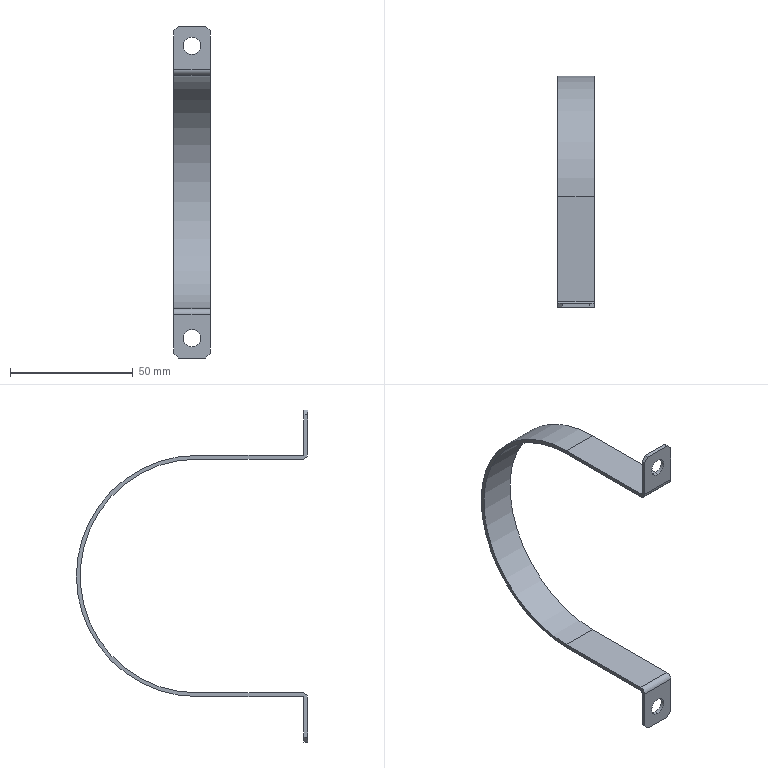Part | SolidWorks | features BaseBody 1 | 1 solid | 26 faces | box 15 x 94 x 135 mm | volume 6112 mm3 | plane 16 | cylinder 10 | commonest cylinder face diameters 7 x4 1.473 x2 4.473 x2 95 x1 98 x1
STEP:
#1=CARTESIAN_POINT('',(0.,0.,-63.));
#2=VERTEX_POINT('',#1);
#3=CARTESIAN_POINT('',(0.,0.,-56.));
#4=VERTEX_POINT('',#3);
#5=CARTESIAN_POINT('',(0.,0.,-59.5));
#6=DIRECTION('',(0.,1.,0.));
#7=DIRECTION('',(0.,0.,-1.));
#8=AXIS2_PLACEMENT_3D('',#5,#6,#7);
#9=CIRCLE('',#8,3.5);
#10=EDGE_CURVE('',#2,#4,#9,.T.);
#11=ORIENTED_EDGE('',*,*,#10,.F.);
#12=CARTESIAN_POINT('',(0.,1.5,-63.));
#13=VERTEX_POINT('',#12);
#14=CARTESIAN_POINT('',(0.,0.,-63.));
#15=DIRECTION('',(0.,1.,0.));
#16=VECTOR('',#15,1000.);
#17=LINE('',#14,#16);
#18=EDGE_CURVE('',#2,#13,#17,.T.);
#19=ORIENTED_EDGE('',*,*,#18,.T.);
#20=CARTESIAN_POINT('',(0.,1.5,-56.));
#21=VERTEX_POINT('',#20);
#22=CARTESIAN_POINT('',(0.,1.5,-59.5));
#23=DIRECTION('',(0.,1.,0.));
#24=DIRECTION('',(0.,0.,-1.));
#25=AXIS2_PLACEMENT_3D('',#22,#23,#24);
#26=CIRCLE('',#25,3.5);
#27=EDGE_CURVE('',#13,#21,#26,.T.);
#28=ORIENTED_EDGE('',*,*,#27,.T.);
#29=CARTESIAN_POINT('',(0.,0.,-56.));
#30=DIRECTION('',(0.,1.,0.));
#31=VECTOR('',#30,1000.);
#32=LINE('',#29,#31);
#33=EDGE_CURVE('',#4,#21,#32,.T.);
#34=ORIENTED_EDGE('',*,*,#33,.F.);
#35=EDGE_LOOP('',(#11,#19,#28,#34));
#36=FACE_OUTER_BOUND('',#35,.T.);
#37=CARTESIAN_POINT('',(0.,0.,-59.5));
#38=DIRECTION('',(0.,1.,0.));
#39=DIRECTION('',(0.,0.,1.));
#40=AXIS2_PLACEMENT_3D('',#37,#38,#39);
#41=CYLINDRICAL_SURFACE('',#40,3.5);
#42=ADVANCED_FACE('',(#36),#41,.F.);
#43=CARTESIAN_POINT('',(0.,0.,56.));
#44=VERTEX_POINT('',#43);
#45=CARTESIAN_POINT('',(0.,0.,63.));
#46=VERTEX_POINT('',#45);
#47=CARTESIAN_POINT('',(0.,0.,59.5));
#48=DIRECTION('',(0.,1.,0.));
#49=DIRECTION('',(0.,0.,1.));
#50=AXIS2_PLACEMENT_3D('',#47,#48,#49);
#51=CIRCLE('',#50,3.5);
#52=EDGE_CURVE('',#44,#46,#51,.T.);
#53=ORIENTED_EDGE('',*,*,#52,.F.);
#54=CARTESIAN_POINT('',(0.,1.5,56.));
#55=VERTEX_POINT('',#54);
#56=CARTESIAN_POINT('',(0.,0.,56.));
#57=DIRECTION('',(0.,1.,0.));
#58=VECTOR('',#57,1000.);
#59=LINE('',#56,#58);
#60=EDGE_CURVE('',#44,#55,#59,.T.);
#61=ORIENTED_EDGE('',*,*,#60,.T.);
#62=CARTESIAN_POINT('',(0.,1.5,63.));
#63=VERTEX_POINT('',#62);
#64=CARTESIAN_POINT('',(0.,1.5,59.5));
#65=DIRECTION('',(0.,1.,0.));
#66=DIRECTION('',(0.,0.,1.));
#67=AXIS2_PLACEMENT_3D('',#64,#65,#66);
#68=CIRCLE('',#67,3.5);
#69=EDGE_CURVE('',#55,#63,#68,.T.);
#70=ORIENTED_EDGE('',*,*,#69,.T.);
#71=CARTESIAN_POINT('',(0.,0.,63.));
#72=DIRECTION('',(0.,1.,0.));
#73=VECTOR('',#72,1000.);
#74=LINE('',#71,#73);
#75=EDGE_CURVE('',#46,#63,#74,.T.);
#76=ORIENTED_EDGE('',*,*,#75,.F.);
#77=EDGE_LOOP('',(#53,#61,#70,#76));
#78=FACE_OUTER_BOUND('',#77,.T.);
#79=CARTESIAN_POINT('',(0.,0.,59.5));
#80=DIRECTION('',(0.,1.,0.));
#81=DIRECTION('',(0.,0.,1.));
#82=AXIS2_PLACEMENT_3D('',#79,#80,#81);
#83=CYLINDRICAL_SURFACE('',#82,3.5);
#84=ADVANCED_FACE('',(#78),#83,.F.);
#85=CARTESIAN_POINT('',(7.5,0.,65.5));
#86=VERTEX_POINT('',#85);
#87=CARTESIAN_POINT('',(5.5,0.,67.5));
#88=VERTEX_POINT('',#87);
#89=CARTESIAN_POINT('',(5.5,0.,67.5));
#90=DIRECTION('',(-0.7071,0.,0.7071));
#91=VECTOR('',#90,1000.);
#92=LINE('',#89,#91);
#93=EDGE_CURVE('',#86,#88,#92,.T.);
#94=ORIENTED_EDGE('',*,*,#93,.F.);
#95=CARTESIAN_POINT('',(7.5,1.5,65.5));
#96=VERTEX_POINT('',#95);
#97=CARTESIAN_POINT('',(7.5,2.237,65.5));
#98=DIRECTION('',(0.,-1.,0.));
#99=VECTOR('',#98,1000.);
#100=LINE('',#97,#99);
#101=EDGE_CURVE('',#96,#86,#100,.T.);
#102=ORIENTED_EDGE('',*,*,#101,.F.);
#103=CARTESIAN_POINT('',(5.5,1.5,67.5));
#104=VERTEX_POINT('',#103);
#105=CARTESIAN_POINT('',(16.5,1.5,56.5));
#106=DIRECTION('',(0.7071,0.,-0.7071));
#107=VECTOR('',#106,1000.);
#108=LINE('',#105,#107);
#109=EDGE_CURVE('',#104,#96,#108,.T.);
#110=ORIENTED_EDGE('',*,*,#109,.F.);
#111=CARTESIAN_POINT('',(5.5,0.,67.5));
#112=DIRECTION('',(0.,1.,0.));
#113=VECTOR('',#112,1000.);
#114=LINE('',#111,#113);
#115=EDGE_CURVE('',#88,#104,#114,.T.);
#116=ORIENTED_EDGE('',*,*,#115,.F.);
#117=EDGE_LOOP('',(#94,#102,#110,#116));
#118=FACE_OUTER_BOUND('',#117,.T.);
#119=CARTESIAN_POINT('',(5.5,0.,67.5));
#120=DIRECTION('',(-0.7071,0.,-0.7071));
#121=DIRECTION('',(-0.7071,0.,0.7071));
#122=AXIS2_PLACEMENT_3D('',#119,#120,#121);
#123=PLANE('',#122);
#124=ADVANCED_FACE('',(#118),#123,.F.);
#125=CARTESIAN_POINT('',(-5.5,0.,67.5));
#126=VERTEX_POINT('',#125);
#127=CARTESIAN_POINT('',(-7.5,0.,65.5));
#128=VERTEX_POINT('',#127);
#129=CARTESIAN_POINT('',(-7.5,0.,65.5));
#130=DIRECTION('',(-0.7071,0.,-0.7071));
#131=VECTOR('',#130,1000.);
#132=LINE('',#129,#131);
#133=EDGE_CURVE('',#126,#128,#132,.T.);
#134=ORIENTED_EDGE('',*,*,#133,.F.);
#135=CARTESIAN_POINT('',(-5.5,1.5,67.5));
#136=VERTEX_POINT('',#135);
#137=CARTESIAN_POINT('',(-5.5,0.,67.5));
#138=DIRECTION('',(0.,-1.,0.));
#139=VECTOR('',#138,1000.);
#140=LINE('',#137,#139);
#141=EDGE_CURVE('',#136,#126,#140,.T.);
#142=ORIENTED_EDGE('',*,*,#141,.F.);
#143=CARTESIAN_POINT('',(-7.5,1.5,65.5));
#144=VERTEX_POINT('',#143);
#145=CARTESIAN_POINT('',(-9.,1.5,64.));
#146=DIRECTION('',(0.7071,0.,0.7071));
#147=VECTOR('',#146,1000.);
#148=LINE('',#145,#147);
#149=EDGE_CURVE('',#144,#136,#148,.T.);
#150=ORIENTED_EDGE('',*,*,#149,.F.);
#151=CARTESIAN_POINT('',(-7.5,1.5,65.5));
#152=DIRECTION('',(0.,1.,0.));
#153=VECTOR('',#152,1000.);
#154=LINE('',#151,#153);
#155=EDGE_CURVE('',#128,#144,#154,.T.);
#156=ORIENTED_EDGE('',*,*,#155,.F.);
#157=EDGE_LOOP('',(#134,#142,#150,#156));
#158=FACE_OUTER_BOUND('',#157,.T.);
#159=CARTESIAN_POINT('',(-7.5,2.237,65.5));
#160=DIRECTION('',(-0.7071,0.,0.7071));
#161=DIRECTION('',(0.,1.,0.));
#162=AXIS2_PLACEMENT_3D('',#159,#160,#161);
#163=PLANE('',#162);
#164=ADVANCED_FACE('',(#158),#163,.T.);
#165=CARTESIAN_POINT('',(7.5,1.5,-65.5));
#166=VERTEX_POINT('',#165);
#167=CARTESIAN_POINT('',(5.5,1.5,-67.5));
#168=VERTEX_POINT('',#167);
#169=CARTESIAN_POINT('',(16.5,1.5,-56.5));
#170=DIRECTION('',(-0.7071,0.,-0.7071));
#171=VECTOR('',#170,1000.);
#172=LINE('',#169,#171);
#173=EDGE_CURVE('',#166,#168,#172,.T.);
#174=ORIENTED_EDGE('',*,*,#173,.F.);
#175=CARTESIAN_POINT('',(7.5,0.,-65.5));
#176=VERTEX_POINT('',#175);
#177=CARTESIAN_POINT('',(7.5,2.237,-65.5));
#178=DIRECTION('',(0.,1.,0.));
#179=VECTOR('',#178,1000.);
#180=LINE('',#177,#179);
#181=EDGE_CURVE('',#176,#166,#180,.T.);
#182=ORIENTED_EDGE('',*,*,#181,.F.);
#183=CARTESIAN_POINT('',(5.5,0.,-67.5));
#184=VERTEX_POINT('',#183);
#185=CARTESIAN_POINT('',(5.5,0.,-67.5));
#186=DIRECTION('',(0.7071,0.,0.7071));
#187=VECTOR('',#186,1000.);
#188=LINE('',#185,#187);
#189=EDGE_CURVE('',#184,#176,#188,.T.);
#190=ORIENTED_EDGE('',*,*,#189,.F.);
#191=CARTESIAN_POINT('',(5.5,1.5,-67.5));
#192=DIRECTION('',(0.,-1.,0.));
#193=VECTOR('',#192,1000.);
#194=LINE('',#191,#193);
#195=EDGE_CURVE('',#168,#184,#194,.T.);
#196=ORIENTED_EDGE('',*,*,#195,.F.);
#197=EDGE_LOOP('',(#174,#182,#190,#196));
#198=FACE_OUTER_BOUND('',#197,.T.);
#199=CARTESIAN_POINT('',(5.5,1.5,-67.5));
#200=DIRECTION('',(-0.7071,0.,0.7071));
#201=DIRECTION('',(0.,1.,0.));
#202=AXIS2_PLACEMENT_3D('',#199,#200,#201);
#203=PLANE('',#202);
#204=ADVANCED_FACE('',(#198),#203,.F.);
#205=CARTESIAN_POINT('',(-5.5,1.5,-67.5));
#206=VERTEX_POINT('',#205);
#207=CARTESIAN_POINT('',(-7.5,1.5,-65.5));
#208=VERTEX_POINT('',#207);
#209=CARTESIAN_POINT('',(-9.,1.5,-64.));
#210=DIRECTION('',(-0.7071,0.,0.7071));
#211=VECTOR('',#210,1000.);
#212=LINE('',#209,#211);
#213=EDGE_CURVE('',#206,#208,#212,.T.);
#214=ORIENTED_EDGE('',*,*,#213,.F.);
#215=CARTESIAN_POINT('',(-5.5,0.,-67.5));
#216=VERTEX_POINT('',#215);
#217=CARTESIAN_POINT('',(-5.5,1.5,-67.5));
#218=DIRECTION('',(0.,1.,0.));
#219=VECTOR('',#218,1000.);
#220=LINE('',#217,#219);
#221=EDGE_CURVE('',#216,#206,#220,.T.);
#222=ORIENTED_EDGE('',*,*,#221,.F.);
#223=CARTESIAN_POINT('',(-7.5,0.,-65.5));
#224=VERTEX_POINT('',#223);
#225=CARTESIAN_POINT('',(-7.5,0.,-65.5));
#226=DIRECTION('',(0.7071,0.,-0.7071));
#227=VECTOR('',#226,1000.);
#228=LINE('',#225,#227);
#229=EDGE_CURVE('',#224,#216,#228,.T.);
#230=ORIENTED_EDGE('',*,*,#229,.F.);
#231=CARTESIAN_POINT('',(-7.5,2.237,-65.5));
#232=DIRECTION('',(0.,-1.,0.));
#233=VECTOR('',#232,1000.);
#234=LINE('',#231,#233);
#235=EDGE_CURVE('',#208,#224,#234,.T.);
#236=ORIENTED_EDGE('',*,*,#235,.F.);
#237=EDGE_LOOP('',(#214,#222,#230,#236));
#238=FACE_OUTER_BOUND('',#237,.T.);
#239=CARTESIAN_POINT('',(-7.5,2.237,-65.5));
#240=DIRECTION('',(0.7071,0.,0.7071));
#241=DIRECTION('',(0.,-1.,0.));
#242=AXIS2_PLACEMENT_3D('',#239,#240,#241);
#243=PLANE('',#242);
#244=ADVANCED_FACE('',(#238),#243,.F.);
#245=CARTESIAN_POINT('',(-7.5,2.237,-47.5));
#246=VERTEX_POINT('',#245);
#247=CARTESIAN_POINT('',(-7.5,0.,-49.737));
#248=VERTEX_POINT('',#247);
#249=CARTESIAN_POINT('',(-7.5,2.237,-49.737));
#250=DIRECTION('',(1.,0.,0.));
#251=DIRECTION('',(0.,0.,1.));
#252=AXIS2_PLACEMENT_3D('',#249,#250,#251);
#253=CIRCLE('',#252,2.237);
#254=EDGE_CURVE('',#246,#248,#253,.T.);
#255=ORIENTED_EDGE('',*,*,#254,.T.);
#256=CARTESIAN_POINT('',(7.5,0.,-49.737));
#257=VERTEX_POINT('',#256);
#258=CARTESIAN_POINT('',(7.5,0.,-49.737));
#259=DIRECTION('',(-1.,0.,0.));
#260=VECTOR('',#259,1000.);
#261=LINE('',#258,#260);
#262=EDGE_CURVE('',#257,#248,#261,.T.);
#263=ORIENTED_EDGE('',*,*,#262,.F.);
#264=CARTESIAN_POINT('',(7.5,2.237,-47.5));
#265=VERTEX_POINT('',#264);
#266=CARTESIAN_POINT('',(7.5,2.237,-49.737));
#267=DIRECTION('',(1.,0.,0.));
#268=DIRECTION('',(0.,0.,1.));
#269=AXIS2_PLACEMENT_3D('',#266,#267,#268);
#270=CIRCLE('',#269,2.237);
#271=EDGE_CURVE('',#265,#257,#270,.T.);
#272=ORIENTED_EDGE('',*,*,#271,.F.);
#273=CARTESIAN_POINT('',(7.5,2.237,-47.5));
#274=DIRECTION('',(-1.,0.,0.));
#275=VECTOR('',#274,1000.);
#276=LINE('',#273,#275);
#277=EDGE_CURVE('',#265,#246,#276,.T.);
#278=ORIENTED_EDGE('',*,*,#277,.T.);
#279=EDGE_LOOP('',(#255,#263,#272,#278));
#280=FACE_OUTER_BOUND('',#279,.T.);
#281=CARTESIAN_POINT('',(7.5,2.237,-49.737));
#282=DIRECTION('',(-1.,0.,0.));
#283=DIRECTION('',(0.,0.,1.));
#284=AXIS2_PLACEMENT_3D('',#281,#282,#283);
#285=CYLINDRICAL_SURFACE('',#284,2.237);
#286=ADVANCED_FACE('',(#280),#285,.T.);
#287=CARTESIAN_POINT('',(-7.5,45.,-47.5));
#288=VERTEX_POINT('',#287);
#289=CARTESIAN_POINT('',(-7.5,45.,-47.5));
#290=DIRECTION('',(0.,-1.,0.));
#291=VECTOR('',#290,1000.);
#292=LINE('',#289,#291);
#293=EDGE_CURVE('',#288,#246,#292,.T.);
#294=ORIENTED_EDGE('',*,*,#293,.T.);
#295=ORIENTED_EDGE('',*,*,#277,.F.);
#296=CARTESIAN_POINT('',(7.5,45.,-47.5));
#297=VERTEX_POINT('',#296);
#298=CARTESIAN_POINT('',(7.5,45.,-47.5));
#299=DIRECTION('',(0.,-1.,0.));
#300=VECTOR('',#299,1000.);
#301=LINE('',#298,#300);
#302=EDGE_CURVE('',#297,#265,#301,.T.);
#303=ORIENTED_EDGE('',*,*,#302,.F.);
#304=CARTESIAN_POINT('',(7.5,45.,-47.5));
#305=DIRECTION('',(-1.,0.,0.));
#306=VECTOR('',#305,1000.);
#307=LINE('',#304,#306);
#308=EDGE_CURVE('',#297,#288,#307,.T.);
#309=ORIENTED_EDGE('',*,*,#308,.T.);
#310=EDGE_LOOP('',(#294,#295,#303,#309));
#311=FACE_OUTER_BOUND('',#310,.T.);
#312=CARTESIAN_POINT('',(7.5,45.,-47.5));
#313=DIRECTION('',(0.,0.,-1.));
#314=DIRECTION('',(0.,-1.,0.));
#315=AXIS2_PLACEMENT_3D('',#312,#313,#314);
#316=PLANE('',#315);
#317=ADVANCED_FACE('',(#311),#316,.F.);
#318=CARTESIAN_POINT('',(-7.5,45.,47.5));
#319=VERTEX_POINT('',#318);
#320=CARTESIAN_POINT('',(-7.5,45.,0.));
#321=DIRECTION('',(-1.,0.,0.));
#322=DIRECTION('',(0.,0.,-1.));
#323=AXIS2_PLACEMENT_3D('',#320,#321,#322);
#324=CIRCLE('',#323,47.5);
#325=EDGE_CURVE('',#319,#288,#324,.T.);
#326=ORIENTED_EDGE('',*,*,#325,.T.);
#327=ORIENTED_EDGE('',*,*,#308,.F.);
#328=CARTESIAN_POINT('',(7.5,45.,47.5));
#329=VERTEX_POINT('',#328);
#330=CARTESIAN_POINT('',(7.5,45.,0.));
#331=DIRECTION('',(-1.,0.,0.));
#332=DIRECTION('',(0.,0.,-1.));
#333=AXIS2_PLACEMENT_3D('',#330,#331,#332);
#334=CIRCLE('',#333,47.5);
#335=EDGE_CURVE('',#329,#297,#334,.T.);
#336=ORIENTED_EDGE('',*,*,#335,.F.);
#337=CARTESIAN_POINT('',(7.5,45.,47.5));
#338=DIRECTION('',(-1.,0.,0.));
#339=VECTOR('',#338,1000.);
#340=LINE('',#337,#339);
#341=EDGE_CURVE('',#329,#319,#340,.T.);
#342=ORIENTED_EDGE('',*,*,#341,.T.);
#343=EDGE_LOOP('',(#326,#327,#336,#342));
#344=FACE_OUTER_BOUND('',#343,.T.);
#345=CARTESIAN_POINT('',(7.5,45.,0.));
#346=DIRECTION('',(-1.,0.,0.));
#347=DIRECTION('',(0.,0.,1.));
#348=AXIS2_PLACEMENT_3D('',#345,#346,#347);
#349=CYLINDRICAL_SURFACE('',#348,47.5);
#350=ADVANCED_FACE('',(#344),#349,.F.);
#351=CARTESIAN_POINT('',(-7.5,2.237,47.5));
#352=VERTEX_POINT('',#351);
#353=CARTESIAN_POINT('',(-7.5,45.,47.5));
#354=DIRECTION('',(0.,1.,0.));
#355=VECTOR('',#354,1000.);
#356=LINE('',#353,#355);
#357=EDGE_CURVE('',#352,#319,#356,.T.);
#358=ORIENTED_EDGE('',*,*,#357,.T.);
#359=ORIENTED_EDGE('',*,*,#341,.F.);
#360=CARTESIAN_POINT('',(7.5,2.237,47.5));
#361=VERTEX_POINT('',#360);
#362=CARTESIAN_POINT('',(7.5,45.,47.5));
#363=DIRECTION('',(0.,1.,0.));
#364=VECTOR('',#363,1000.);
#365=LINE('',#362,#364);
#366=EDGE_CURVE('',#361,#329,#365,.T.);
#367=ORIENTED_EDGE('',*,*,#366,.F.);
#368=CARTESIAN_POINT('',(7.5,2.237,47.5));
#369=DIRECTION('',(-1.,0.,0.));
#370=VECTOR('',#369,1000.);
#371=LINE('',#368,#370);
#372=EDGE_CURVE('',#361,#352,#371,.T.);
#373=ORIENTED_EDGE('',*,*,#372,.T.);
#374=EDGE_LOOP('',(#358,#359,#367,#373));
#375=FACE_OUTER_BOUND('',#374,.T.);
#376=CARTESIAN_POINT('',(7.5,45.,47.5));
#377=DIRECTION('',(0.,0.,1.));
#378=DIRECTION('',(1.,0.,0.));
#379=AXIS2_PLACEMENT_3D('',#376,#377,#378);
#380=PLANE('',#379);
#381=ADVANCED_FACE('',(#375),#380,.F.);
#382=CARTESIAN_POINT('',(-7.5,0.,49.737));
#383=VERTEX_POINT('',#382);
#384=CARTESIAN_POINT('',(-7.5,2.237,49.737));
#385=DIRECTION('',(1.,0.,0.));
#386=DIRECTION('',(0.,0.,1.));
#387=AXIS2_PLACEMENT_3D('',#384,#385,#386);
#388=CIRCLE('',#387,2.237);
#389=EDGE_CURVE('',#383,#352,#388,.T.);
#390=ORIENTED_EDGE('',*,*,#389,.T.);
#391=ORIENTED_EDGE('',*,*,#372,.F.);
#392=CARTESIAN_POINT('',(7.5,0.,49.737));
#393=VERTEX_POINT('',#392);
#394=CARTESIAN_POINT('',(7.5,2.237,49.737));
#395=DIRECTION('',(1.,0.,0.));
#396=DIRECTION('',(0.,0.,1.));
#397=AXIS2_PLACEMENT_3D('',#394,#395,#396);
#398=CIRCLE('',#397,2.237);
#399=EDGE_CURVE('',#393,#361,#398,.T.);
#400=ORIENTED_EDGE('',*,*,#399,.F.);
#401=CARTESIAN_POINT('',(7.5,0.,49.737));
#402=DIRECTION('',(-1.,0.,0.));
#403=VECTOR('',#402,1000.);
#404=LINE('',#401,#403);
#405=EDGE_CURVE('',#393,#383,#404,.T.);
#406=ORIENTED_EDGE('',*,*,#405,.T.);
#407=EDGE_LOOP('',(#390,#391,#400,#406));
#408=FACE_OUTER_BOUND('',#407,.T.);
#409=CARTESIAN_POINT('',(7.5,2.237,49.737));
#410=DIRECTION('',(-1.,0.,0.));
#411=DIRECTION('',(0.,0.,1.));
#412=AXIS2_PLACEMENT_3D('',#409,#410,#411);
#413=CYLINDRICAL_SURFACE('',#412,2.237);
#414=ADVANCED_FACE('',(#408),#413,.T.);
#415=CARTESIAN_POINT('',(0.,0.,59.5));
#416=DIRECTION('',(0.,1.,0.));
#417=DIRECTION('',(0.,0.,1.));
#418=AXIS2_PLACEMENT_3D('',#415,#416,#417);
#419=CIRCLE('',#418,3.5);
#420=EDGE_CURVE('',#46,#44,#419,.T.);
#421=ORIENTED_EDGE('',*,*,#420,.T.);
#422=ORIENTED_EDGE('',*,*,#52,.T.);
#423=EDGE_LOOP('',(#421,#422));
#424=FACE_BOUND('',#423,.T.);
#425=CARTESIAN_POINT('',(7.5,0.,67.5));
#426=DIRECTION('',(-1.,0.,0.));
#427=VECTOR('',#426,1000.);
#428=LINE('',#425,#427);
#429=EDGE_CURVE('',#88,#126,#428,.T.);
#430=ORIENTED_EDGE('',*,*,#429,.T.);
#431=ORIENTED_EDGE('',*,*,#133,.T.);
#432=CARTESIAN_POINT('',(-7.5,0.,47.5));
#433=DIRECTION('',(0.,0.,-1.));
#434=VECTOR('',#433,1000.);
#435=LINE('',#432,#434);
#436=EDGE_CURVE('',#128,#383,#435,.T.);
#437=ORIENTED_EDGE('',*,*,#436,.T.);
#438=ORIENTED_EDGE('',*,*,#405,.F.);
#439=CARTESIAN_POINT('',(7.5,0.,47.5));
#440=DIRECTION('',(0.,0.,-1.));
#441=VECTOR('',#440,1000.);
#442=LINE('',#439,#441);
#443=EDGE_CURVE('',#86,#393,#442,.T.);
#444=ORIENTED_EDGE('',*,*,#443,.F.);
#445=ORIENTED_EDGE('',*,*,#93,.T.);
#446=EDGE_LOOP('',(#430,#431,#437,#438,#444,#445));
#447=FACE_OUTER_BOUND('',#446,.T.);
#448=CARTESIAN_POINT('',(7.5,0.,47.5));
#449=DIRECTION('',(0.,1.,0.));
#450=DIRECTION('',(0.,0.,-1.));
#451=AXIS2_PLACEMENT_3D('',#448,#449,#450);
#452=PLANE('',#451);
#453=ADVANCED_FACE('',(#424,#447),#452,.F.);
#454=CARTESIAN_POINT('',(7.5,1.5,67.5));
#455=DIRECTION('',(-1.,0.,0.));
#456=VECTOR('',#455,1000.);
#457=LINE('',#454,#456);
#458=EDGE_CURVE('',#104,#136,#457,.T.);
#459=ORIENTED_EDGE('',*,*,#458,.T.);
#460=ORIENTED_EDGE('',*,*,#141,.T.);
#461=ORIENTED_EDGE('',*,*,#429,.F.);
#462=ORIENTED_EDGE('',*,*,#115,.T.);
#463=EDGE_LOOP('',(#459,#460,#461,#462));
#464=FACE_OUTER_BOUND('',#463,.T.);
#465=CARTESIAN_POINT('',(7.5,0.,67.5));
#466=DIRECTION('',(0.,0.,1.));
#467=DIRECTION('',(1.,0.,0.));
#468=AXIS2_PLACEMENT_3D('',#465,#466,#467);
#469=PLANE('',#468);
#470=ADVANCED_FACE('',(#464),#469,.T.);
#471=CARTESIAN_POINT('',(0.,1.5,59.5));
#472=DIRECTION('',(0.,1.,0.));
#473=DIRECTION('',(0.,0.,1.));
#474=AXIS2_PLACEMENT_3D('',#471,#472,#473);
#475=CIRCLE('',#474,3.5);
#476=EDGE_CURVE('',#63,#55,#475,.T.);
#477=ORIENTED_EDGE('',*,*,#476,.F.);
#478=ORIENTED_EDGE('',*,*,#69,.F.);
#479=EDGE_LOOP('',(#477,#478));
#480=FACE_BOUND('',#479,.T.);
#481=CARTESIAN_POINT('',(-7.5,1.5,49.737));
#482=VERTEX_POINT('',#481);
#483=CARTESIAN_POINT('',(-7.5,1.5,47.5));
#484=DIRECTION('',(0.,0.,-1.));
#485=VECTOR('',#484,1000.);
#486=LINE('',#483,#485);
#487=EDGE_CURVE('',#144,#482,#486,.T.);
#488=ORIENTED_EDGE('',*,*,#487,.F.);
#489=ORIENTED_EDGE('',*,*,#149,.T.);
#490=ORIENTED_EDGE('',*,*,#458,.F.);
#491=ORIENTED_EDGE('',*,*,#109,.T.);
#492=CARTESIAN_POINT('',(7.5,1.5,49.737));
#493=VERTEX_POINT('',#492);
#494=CARTESIAN_POINT('',(7.5,1.5,47.5));
#495=DIRECTION('',(0.,0.,-1.));
#496=VECTOR('',#495,1000.);
#497=LINE('',#494,#496);
#498=EDGE_CURVE('',#96,#493,#497,.T.);
#499=ORIENTED_EDGE('',*,*,#498,.T.);
#500=CARTESIAN_POINT('',(7.5,1.5,49.737));
#501=DIRECTION('',(-1.,0.,0.));
#502=VECTOR('',#501,1000.);
#503=LINE('',#500,#502);
#504=EDGE_CURVE('',#493,#482,#503,.T.);
#505=ORIENTED_EDGE('',*,*,#504,.T.);
#506=EDGE_LOOP('',(#488,#489,#490,#491,#499,#505));
#507=FACE_OUTER_BOUND('',#506,.T.);
#508=CARTESIAN_POINT('',(7.5,1.5,47.5));
#509=DIRECTION('',(0.,1.,0.));
#510=DIRECTION('',(0.,0.,-1.));
#511=AXIS2_PLACEMENT_3D('',#508,#509,#510);
#512=PLANE('',#511);
#513=ADVANCED_FACE('',(#480,#507),#512,.T.);
#514=CARTESIAN_POINT('',(-7.5,2.237,49.));
#515=VERTEX_POINT('',#514);
#516=CARTESIAN_POINT('',(-7.5,2.237,49.737));
#517=DIRECTION('',(1.,0.,0.));
#518=DIRECTION('',(0.,0.,-1.));
#519=AXIS2_PLACEMENT_3D('',#516,#517,#518);
#520=CIRCLE('',#519,0.7366);
#521=EDGE_CURVE('',#482,#515,#520,.T.);
#522=ORIENTED_EDGE('',*,*,#521,.F.);
#523=ORIENTED_EDGE('',*,*,#504,.F.);
#524=CARTESIAN_POINT('',(7.5,2.237,49.));
#525=VERTEX_POINT('',#524);
#526=CARTESIAN_POINT('',(7.5,2.237,49.737));
#527=DIRECTION('',(1.,0.,0.));
#528=DIRECTION('',(0.,0.,-1.));
#529=AXIS2_PLACEMENT_3D('',#526,#527,#528);
#530=CIRCLE('',#529,0.7366);
#531=EDGE_CURVE('',#493,#525,#530,.T.);
#532=ORIENTED_EDGE('',*,*,#531,.T.);
#533=CARTESIAN_POINT('',(7.5,2.237,49.));
#534=DIRECTION('',(-1.,0.,0.));
#535=VECTOR('',#534,1000.);
#536=LINE('',#533,#535);
#537=EDGE_CURVE('',#525,#515,#536,.T.);
#538=ORIENTED_EDGE('',*,*,#537,.T.);
#539=EDGE_LOOP('',(#522,#523,#532,#538));
#540=FACE_OUTER_BOUND('',#539,.T.);
#541=CARTESIAN_POINT('',(7.5,2.237,49.737));
#542=DIRECTION('',(-1.,0.,0.));
#543=DIRECTION('',(0.,0.,1.));
#544=AXIS2_PLACEMENT_3D('',#541,#542,#543);
#545=CYLINDRICAL_SURFACE('',#544,0.7366);
#546=ADVANCED_FACE('',(#540),#545,.F.);
#547=CARTESIAN_POINT('',(-7.5,45.,49.));
#548=VERTEX_POINT('',#547);
#549=CARTESIAN_POINT('',(-7.5,45.,49.));
#550=DIRECTION('',(0.,1.,0.));
#551=VECTOR('',#550,1000.);
#552=LINE('',#549,#551);
#553=EDGE_CURVE('',#515,#548,#552,.T.);
#554=ORIENTED_EDGE('',*,*,#553,.F.);
#555=ORIENTED_EDGE('',*,*,#537,.F.);
#556=CARTESIAN_POINT('',(7.5,45.,49.));
#557=VERTEX_POINT('',#556);
#558=CARTESIAN_POINT('',(7.5,45.,49.));
#559=DIRECTION('',(0.,1.,0.));
#560=VECTOR('',#559,1000.);
#561=LINE('',#558,#560);
#562=EDGE_CURVE('',#525,#557,#561,.T.);
#563=ORIENTED_EDGE('',*,*,#562,.T.);
#564=CARTESIAN_POINT('',(7.5,45.,49.));
#565=DIRECTION('',(-1.,0.,0.));
#566=VECTOR('',#565,1000.);
#567=LINE('',#564,#566);
#568=EDGE_CURVE('',#557,#548,#567,.T.);
#569=ORIENTED_EDGE('',*,*,#568,.T.);
#570=EDGE_LOOP('',(#554,#555,#563,#569));
#571=FACE_OUTER_BOUND('',#570,.T.);
#572=CARTESIAN_POINT('',(7.5,45.,49.));
#573=DIRECTION('',(0.,0.,1.));
#574=DIRECTION('',(1.,0.,0.));
#575=AXIS2_PLACEMENT_3D('',#572,#573,#574);
#576=PLANE('',#575);
#577=ADVANCED_FACE('',(#571),#576,.T.);
#578=CARTESIAN_POINT('',(-7.5,45.,-49.));
#579=VERTEX_POINT('',#578);
#580=CARTESIAN_POINT('',(-7.5,45.,0.));
#581=DIRECTION('',(-1.,0.,0.));
#582=DIRECTION('',(0.,0.,-1.));
#583=AXIS2_PLACEMENT_3D('',#580,#581,#582);
#584=CIRCLE('',#583,49.);
#585=EDGE_CURVE('',#548,#579,#584,.T.);
#586=ORIENTED_EDGE('',*,*,#585,.F.);
#587=ORIENTED_EDGE('',*,*,#568,.F.);
#588=CARTESIAN_POINT('',(7.5,45.,-49.));
#589=VERTEX_POINT('',#588);
#590=CARTESIAN_POINT('',(7.5,45.,0.));
#591=DIRECTION('',(-1.,0.,0.));
#592=DIRECTION('',(0.,0.,-1.));
#593=AXIS2_PLACEMENT_3D('',#590,#591,#592);
#594=CIRCLE('',#593,49.);
#595=EDGE_CURVE('',#557,#589,#594,.T.);
#596=ORIENTED_EDGE('',*,*,#595,.T.);
#597=CARTESIAN_POINT('',(7.5,45.,-49.));
#598=DIRECTION('',(-1.,0.,0.));
#599=VECTOR('',#598,1000.);
#600=LINE('',#597,#599);
#601=EDGE_CURVE('',#589,#579,#600,.T.);
#602=ORIENTED_EDGE('',*,*,#601,.T.);
#603=EDGE_LOOP('',(#586,#587,#596,#602));
#604=FACE_OUTER_BOUND('',#603,.T.);
#605=CARTESIAN_POINT('',(7.5,45.,0.));
#606=DIRECTION('',(-1.,0.,0.));
#607=DIRECTION('',(0.,0.,1.));
#608=AXIS2_PLACEMENT_3D('',#605,#606,#607);
#609=CYLINDRICAL_SURFACE('',#608,49.);
#610=ADVANCED_FACE('',(#604),#609,.T.);
#611=CARTESIAN_POINT('',(-7.5,2.237,-49.));
#612=VERTEX_POINT('',#611);
#613=CARTESIAN_POINT('',(-7.5,45.,-49.));
#614=DIRECTION('',(0.,-1.,0.));
#615=VECTOR('',#614,1000.);
#616=LINE('',#613,#615);
#617=EDGE_CURVE('',#579,#612,#616,.T.);
#618=ORIENTED_EDGE('',*,*,#617,.F.);
#619=ORIENTED_EDGE('',*,*,#601,.F.);
#620=CARTESIAN_POINT('',(7.5,2.237,-49.));
#621=VERTEX_POINT('',#620);
#622=CARTESIAN_POINT('',(7.5,45.,-49.));
#623=DIRECTION('',(0.,-1.,0.));
#624=VECTOR('',#623,1000.);
#625=LINE('',#622,#624);
#626=EDGE_CURVE('',#589,#621,#625,.T.);
#627=ORIENTED_EDGE('',*,*,#626,.T.);
#628=CARTESIAN_POINT('',(7.5,2.237,-49.));
#629=DIRECTION('',(-1.,0.,0.));
#630=VECTOR('',#629,1000.);
#631=LINE('',#628,#630);
#632=EDGE_CURVE('',#621,#612,#631,.T.);
#633=ORIENTED_EDGE('',*,*,#632,.T.);
#634=EDGE_LOOP('',(#618,#619,#627,#633));
#635=FACE_OUTER_BOUND('',#634,.T.);
#636=CARTESIAN_POINT('',(7.5,45.,-49.));
#637=DIRECTION('',(0.,0.,-1.));
#638=DIRECTION('',(0.,-1.,0.));
#639=AXIS2_PLACEMENT_3D('',#636,#637,#638);
#640=PLANE('',#639);
#641=ADVANCED_FACE('',(#635),#640,.T.);
#642=CARTESIAN_POINT('',(-7.5,1.5,-49.737));
#643=VERTEX_POINT('',#642);
#644=CARTESIAN_POINT('',(-7.5,2.237,-49.737));
#645=DIRECTION('',(1.,0.,0.));
#646=DIRECTION('',(0.,0.,-1.));
#647=AXIS2_PLACEMENT_3D('',#644,#645,#646);
#648=CIRCLE('',#647,0.7366);
#649=EDGE_CURVE('',#612,#643,#648,.T.);
#650=ORIENTED_EDGE('',*,*,#649,.F.);
#651=ORIENTED_EDGE('',*,*,#632,.F.);
#652=CARTESIAN_POINT('',(7.5,1.5,-49.737));
#653=VERTEX_POINT('',#652);
#654=CARTESIAN_POINT('',(7.5,2.237,-49.737));
#655=DIRECTION('',(1.,0.,0.));
#656=DIRECTION('',(0.,0.,-1.));
#657=AXIS2_PLACEMENT_3D('',#654,#655,#656);
#658=CIRCLE('',#657,0.7366);
#659=EDGE_CURVE('',#621,#653,#658,.T.);
#660=ORIENTED_EDGE('',*,*,#659,.T.);
#661=CARTESIAN_POINT('',(7.5,1.5,-49.737));
#662=DIRECTION('',(-1.,0.,0.));
#663=VECTOR('',#662,1000.);
#664=LINE('',#661,#663);
#665=EDGE_CURVE('',#653,#643,#664,.T.);
#666=ORIENTED_EDGE('',*,*,#665,.T.);
#667=EDGE_LOOP('',(#650,#651,#660,#666));
#668=FACE_OUTER_BOUND('',#667,.T.);
#669=CARTESIAN_POINT('',(7.5,2.237,-49.737));
#670=DIRECTION('',(-1.,0.,0.));
#671=DIRECTION('',(0.,0.,1.));
#672=AXIS2_PLACEMENT_3D('',#669,#670,#671);
#673=CYLINDRICAL_SURFACE('',#672,0.7366);
#674=ADVANCED_FACE('',(#668),#673,.F.);
#675=CARTESIAN_POINT('',(0.,1.5,-59.5));
#676=DIRECTION('',(0.,1.,0.));
#677=DIRECTION('',(0.,0.,-1.));
#678=AXIS2_PLACEMENT_3D('',#675,#676,#677);
#679=CIRCLE('',#678,3.5);
#680=EDGE_CURVE('',#21,#13,#679,.T.);
#681=ORIENTED_EDGE('',*,*,#680,.F.);
#682=ORIENTED_EDGE('',*,*,#27,.F.);
#683=EDGE_LOOP('',(#681,#682));
#684=FACE_BOUND('',#683,.T.);
#685=CARTESIAN_POINT('',(7.5,1.5,-67.5));
#686=DIRECTION('',(-1.,0.,0.));
#687=VECTOR('',#686,1000.);
#688=LINE('',#685,#687);
#689=EDGE_CURVE('',#168,#206,#688,.T.);
#690=ORIENTED_EDGE('',*,*,#689,.T.);
#691=ORIENTED_EDGE('',*,*,#213,.T.);
#692=CARTESIAN_POINT('',(-7.5,1.5,-47.5));
#693=DIRECTION('',(0.,0.,-1.));
#694=VECTOR('',#693,1000.);
#695=LINE('',#692,#694);
#696=EDGE_CURVE('',#643,#208,#695,.T.);
#697=ORIENTED_EDGE('',*,*,#696,.F.);
#698=ORIENTED_EDGE('',*,*,#665,.F.);
#699=CARTESIAN_POINT('',(7.5,1.5,-47.5));
#700=DIRECTION('',(0.,0.,-1.));
#701=VECTOR('',#700,1000.);
#702=LINE('',#699,#701);
#703=EDGE_CURVE('',#653,#166,#702,.T.);
#704=ORIENTED_EDGE('',*,*,#703,.T.);
#705=ORIENTED_EDGE('',*,*,#173,.T.);
#706=EDGE_LOOP('',(#690,#691,#697,#698,#704,#705));
#707=FACE_OUTER_BOUND('',#706,.T.);
#708=CARTESIAN_POINT('',(7.5,1.5,-47.5));
#709=DIRECTION('',(0.,1.,0.));
#710=DIRECTION('',(0.,0.,-1.));
#711=AXIS2_PLACEMENT_3D('',#708,#709,#710);
#712=PLANE('',#711);
#713=ADVANCED_FACE('',(#684,#707),#712,.T.);
#714=CARTESIAN_POINT('',(7.5,0.,-67.5));
#715=DIRECTION('',(-1.,0.,0.));
#716=VECTOR('',#715,1000.);
#717=LINE('',#714,#716);
#718=EDGE_CURVE('',#184,#216,#717,.T.);
#719=ORIENTED_EDGE('',*,*,#718,.T.);
#720=ORIENTED_EDGE('',*,*,#221,.T.);
#721=ORIENTED_EDGE('',*,*,#689,.F.);
#722=ORIENTED_EDGE('',*,*,#195,.T.);
#723=EDGE_LOOP('',(#719,#720,#721,#722));
#724=FACE_OUTER_BOUND('',#723,.T.);
#725=CARTESIAN_POINT('',(7.5,1.5,-67.5));
#726=DIRECTION('',(0.,0.,-1.));
#727=DIRECTION('',(0.,-1.,0.));
#728=AXIS2_PLACEMENT_3D('',#725,#726,#727);
#729=PLANE('',#728);
#730=ADVANCED_FACE('',(#724),#729,.T.);
#731=CARTESIAN_POINT('',(0.,0.,-59.5));
#732=DIRECTION('',(0.,1.,0.));
#733=DIRECTION('',(0.,0.,-1.));
#734=AXIS2_PLACEMENT_3D('',#731,#732,#733);
#735=CIRCLE('',#734,3.5);
#736=EDGE_CURVE('',#4,#2,#735,.T.);
#737=ORIENTED_EDGE('',*,*,#736,.T.);
#738=ORIENTED_EDGE('',*,*,#10,.T.);
#739=EDGE_LOOP('',(#737,#738));
#740=FACE_BOUND('',#739,.T.);
#741=CARTESIAN_POINT('',(-7.5,0.,-47.5));
#742=DIRECTION('',(0.,0.,-1.));
#743=VECTOR('',#742,1000.);
#744=LINE('',#741,#743);
#745=EDGE_CURVE('',#248,#224,#744,.T.);
#746=ORIENTED_EDGE('',*,*,#745,.T.);
#747=ORIENTED_EDGE('',*,*,#229,.T.);
#748=ORIENTED_EDGE('',*,*,#718,.F.);
#749=ORIENTED_EDGE('',*,*,#189,.T.);
#750=CARTESIAN_POINT('',(7.5,0.,-47.5));
#751=DIRECTION('',(0.,0.,-1.));
#752=VECTOR('',#751,1000.);
#753=LINE('',#750,#752);
#754=EDGE_CURVE('',#257,#176,#753,.T.);
#755=ORIENTED_EDGE('',*,*,#754,.F.);
#756=ORIENTED_EDGE('',*,*,#262,.T.);
#757=EDGE_LOOP('',(#746,#747,#748,#749,#755,#756));
#758=FACE_OUTER_BOUND('',#757,.T.);
#759=CARTESIAN_POINT('',(7.5,0.,-47.5));
#760=DIRECTION('',(0.,1.,0.));
#761=DIRECTION('',(0.,0.,-1.));
#762=AXIS2_PLACEMENT_3D('',#759,#760,#761);
#763=PLANE('',#762);
#764=ADVANCED_FACE('',(#740,#758),#763,.F.);
#765=ORIENTED_EDGE('',*,*,#585,.T.);
#766=ORIENTED_EDGE('',*,*,#617,.T.);
#767=ORIENTED_EDGE('',*,*,#649,.T.);
#768=ORIENTED_EDGE('',*,*,#696,.T.);
#769=ORIENTED_EDGE('',*,*,#235,.T.);
#770=ORIENTED_EDGE('',*,*,#745,.F.);
#771=ORIENTED_EDGE('',*,*,#254,.F.);
#772=ORIENTED_EDGE('',*,*,#293,.F.);
#773=ORIENTED_EDGE('',*,*,#325,.F.);
#774=ORIENTED_EDGE('',*,*,#357,.F.);
#775=ORIENTED_EDGE('',*,*,#389,.F.);
#776=ORIENTED_EDGE('',*,*,#436,.F.);
#777=ORIENTED_EDGE('',*,*,#155,.T.);
#778=ORIENTED_EDGE('',*,*,#487,.T.);
#779=ORIENTED_EDGE('',*,*,#521,.T.);
#780=ORIENTED_EDGE('',*,*,#553,.T.);
#781=EDGE_LOOP('',(#765,#766,#767,#768,#769,#770,#771,#772,#773,#774,#775,#776,#777,#778,#779,#780));
#782=FACE_OUTER_BOUND('',#781,.T.);
#783=CARTESIAN_POINT('',(-7.5,45.,-47.5));
#784=DIRECTION('',(-1.,0.,0.));
#785=DIRECTION('',(0.,0.,1.));
#786=AXIS2_PLACEMENT_3D('',#783,#784,#785);
#787=PLANE('',#786);
#788=ADVANCED_FACE('',(#782),#787,.T.);
#789=ORIENTED_EDGE('',*,*,#595,.F.);
#790=ORIENTED_EDGE('',*,*,#562,.F.);
#791=ORIENTED_EDGE('',*,*,#531,.F.);
#792=ORIENTED_EDGE('',*,*,#498,.F.);
#793=ORIENTED_EDGE('',*,*,#101,.T.);
#794=ORIENTED_EDGE('',*,*,#443,.T.);
#795=ORIENTED_EDGE('',*,*,#399,.T.);
#796=ORIENTED_EDGE('',*,*,#366,.T.);
#797=ORIENTED_EDGE('',*,*,#335,.T.);
#798=ORIENTED_EDGE('',*,*,#302,.T.);
#799=ORIENTED_EDGE('',*,*,#271,.T.);
#800=ORIENTED_EDGE('',*,*,#754,.T.);
#801=ORIENTED_EDGE('',*,*,#181,.T.);
#802=ORIENTED_EDGE('',*,*,#703,.F.);
#803=ORIENTED_EDGE('',*,*,#659,.F.);
#804=ORIENTED_EDGE('',*,*,#626,.F.);
#805=EDGE_LOOP('',(#789,#790,#791,#792,#793,#794,#795,#796,#797,#798,#799,#800,#801,#802,#803,#804));
#806=FACE_OUTER_BOUND('',#805,.T.);
#807=CARTESIAN_POINT('',(7.5,45.,47.5));
#808=DIRECTION('',(1.,0.,0.));
#809=DIRECTION('',(0.,1.,0.));
#810=AXIS2_PLACEMENT_3D('',#807,#808,#809);
#811=PLANE('',#810);
#812=ADVANCED_FACE('',(#806),#811,.T.);
#813=ORIENTED_EDGE('',*,*,#60,.F.);
#814=ORIENTED_EDGE('',*,*,#420,.F.);
#815=ORIENTED_EDGE('',*,*,#75,.T.);
#816=ORIENTED_EDGE('',*,*,#476,.T.);
#817=EDGE_LOOP('',(#813,#814,#815,#816));
#818=FACE_OUTER_BOUND('',#817,.T.);
#819=CARTESIAN_POINT('',(0.,0.,59.5));
#820=DIRECTION('',(0.,1.,0.));
#821=DIRECTION('',(0.,0.,1.));
#822=AXIS2_PLACEMENT_3D('',#819,#820,#821);
#823=CYLINDRICAL_SURFACE('',#822,3.5);
#824=ADVANCED_FACE('',(#818),#823,.F.);
#825=ORIENTED_EDGE('',*,*,#18,.F.);
#826=ORIENTED_EDGE('',*,*,#736,.F.);
#827=ORIENTED_EDGE('',*,*,#33,.T.);
#828=ORIENTED_EDGE('',*,*,#680,.T.);
#829=EDGE_LOOP('',(#825,#826,#827,#828));
#830=FACE_OUTER_BOUND('',#829,.T.);
#831=CARTESIAN_POINT('',(0.,0.,-59.5));
#832=DIRECTION('',(0.,1.,0.));
#833=DIRECTION('',(0.,0.,1.));
#834=AXIS2_PLACEMENT_3D('',#831,#832,#833);
#835=CYLINDRICAL_SURFACE('',#834,3.5);
#836=ADVANCED_FACE('',(#830),#835,.F.);
#837=CLOSED_SHELL('',(#42,#84,#124,#164,#204,#244,#286,#317,#350,#381,#414,#453,#470,#513,#546,#577,#610,#641,#674,#713,#730,#764,#788,#812,#824,#836));
#838=MANIFOLD_SOLID_BREP('',#837);
#839=CARTESIAN_POINT('',(0.,0.,0.));
#840=DIRECTION('',(0.,0.,1.));
#841=DIRECTION('',(1.,0.,0.));
#842=AXIS2_PLACEMENT_3D('',#839,#840,#841);
#843=(LENGTH_UNIT()NAMED_UNIT(*)SI_UNIT(.MILLI.,.METRE.));
#844=UNCERTAINTY_MEASURE_WITH_UNIT(LENGTH_MEASURE(0.00001),#843,'','');
#845=(NAMED_UNIT(*)PLANE_ANGLE_UNIT()SI_UNIT($,.RADIAN.));
#846=(NAMED_UNIT(*)SI_UNIT($,.STERADIAN.)SOLID_ANGLE_UNIT());
#847=(GEOMETRIC_REPRESENTATION_CONTEXT(3)GLOBAL_UNCERTAINTY_ASSIGNED_CONTEXT((#844))GLOBAL_UNIT_ASSIGNED_CONTEXT((#843,#845,#846))REPRESENTATION_CONTEXT('',''));
#848=ADVANCED_BREP_SHAPE_REPRESENTATION('',(#838,#842),#847);